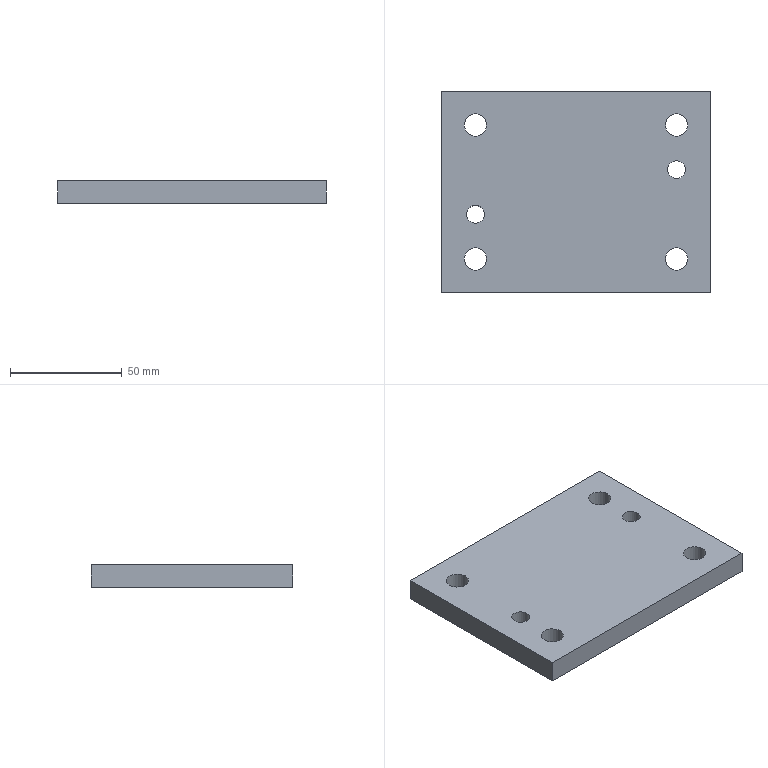Part | NX | features DATUM_CSYS 1, EXTRUDE 1 | 1 solid | 12 faces | box 120 x 90 x 10 mm | volume 103853 mm3 | plane 6 | cylinder 6 | commonest cylinder face diameters 10 x4 8 x2
STEP:
#1=CARTESIAN_POINT('',(60.,-45.,0.));
#2=VERTEX_POINT('',#1);
#3=CARTESIAN_POINT('',(60.,45.,0.));
#4=VERTEX_POINT('',#3);
#5=CARTESIAN_POINT('',(60.,-45.,0.));
#6=DIRECTION('',(0.,1.,0.));
#7=VECTOR('',#6,1000.);
#8=LINE('',#5,#7);
#9=EDGE_CURVE('',#2,#4,#8,.T.);
#10=ORIENTED_EDGE('',*,*,#9,.T.);
#11=CARTESIAN_POINT('',(60.,45.,10.));
#12=VERTEX_POINT('',#11);
#13=CARTESIAN_POINT('',(60.,45.,10.));
#14=DIRECTION('',(0.,0.,-1.));
#15=VECTOR('',#14,1000.);
#16=LINE('',#13,#15);
#17=EDGE_CURVE('',#12,#4,#16,.T.);
#18=ORIENTED_EDGE('',*,*,#17,.F.);
#19=CARTESIAN_POINT('',(60.,-45.,10.));
#20=VERTEX_POINT('',#19);
#21=CARTESIAN_POINT('',(60.,-45.,10.));
#22=DIRECTION('',(0.,1.,0.));
#23=VECTOR('',#22,1000.);
#24=LINE('',#21,#23);
#25=EDGE_CURVE('',#20,#12,#24,.T.);
#26=ORIENTED_EDGE('',*,*,#25,.F.);
#27=CARTESIAN_POINT('',(60.,-45.,10.));
#28=DIRECTION('',(0.,0.,-1.));
#29=VECTOR('',#28,1000.);
#30=LINE('',#27,#29);
#31=EDGE_CURVE('',#20,#2,#30,.T.);
#32=ORIENTED_EDGE('',*,*,#31,.T.);
#33=EDGE_LOOP('',(#10,#18,#26,#32));
#34=FACE_BOUND('',#33,.T.);
#35=CARTESIAN_POINT('',(60.,-45.,10.));
#36=DIRECTION('',(-1.,0.,0.));
#37=DIRECTION('',(0.,0.,1.));
#38=AXIS2_PLACEMENT_3D('',#35,#36,#37);
#39=PLANE('',#38);
#40=ADVANCED_FACE('',(#34),#39,.F.);
#41=CARTESIAN_POINT('',(-60.,45.,0.));
#42=VERTEX_POINT('',#41);
#43=CARTESIAN_POINT('',(60.,45.,0.));
#44=DIRECTION('',(-1.,0.,0.));
#45=VECTOR('',#44,1000.);
#46=LINE('',#43,#45);
#47=EDGE_CURVE('',#4,#42,#46,.T.);
#48=ORIENTED_EDGE('',*,*,#47,.T.);
#49=CARTESIAN_POINT('',(-60.,45.,10.));
#50=VERTEX_POINT('',#49);
#51=CARTESIAN_POINT('',(-60.,45.,10.));
#52=DIRECTION('',(0.,0.,-1.));
#53=VECTOR('',#52,1000.);
#54=LINE('',#51,#53);
#55=EDGE_CURVE('',#50,#42,#54,.T.);
#56=ORIENTED_EDGE('',*,*,#55,.F.);
#57=CARTESIAN_POINT('',(60.,45.,10.));
#58=DIRECTION('',(-1.,0.,0.));
#59=VECTOR('',#58,1000.);
#60=LINE('',#57,#59);
#61=EDGE_CURVE('',#12,#50,#60,.T.);
#62=ORIENTED_EDGE('',*,*,#61,.F.);
#63=ORIENTED_EDGE('',*,*,#17,.T.);
#64=EDGE_LOOP('',(#48,#56,#62,#63));
#65=FACE_BOUND('',#64,.T.);
#66=CARTESIAN_POINT('',(60.,45.,10.));
#67=DIRECTION('',(0.,-1.,0.));
#68=DIRECTION('',(0.,0.,-1.));
#69=AXIS2_PLACEMENT_3D('',#66,#67,#68);
#70=PLANE('',#69);
#71=ADVANCED_FACE('',(#65),#70,.F.);
#72=CARTESIAN_POINT('',(-60.,-45.,0.));
#73=VERTEX_POINT('',#72);
#74=CARTESIAN_POINT('',(-60.,45.,0.));
#75=DIRECTION('',(0.,-1.,0.));
#76=VECTOR('',#75,1000.);
#77=LINE('',#74,#76);
#78=EDGE_CURVE('',#42,#73,#77,.T.);
#79=ORIENTED_EDGE('',*,*,#78,.T.);
#80=CARTESIAN_POINT('',(-60.,-45.,10.));
#81=VERTEX_POINT('',#80);
#82=CARTESIAN_POINT('',(-60.,-45.,10.));
#83=DIRECTION('',(0.,0.,-1.));
#84=VECTOR('',#83,1000.);
#85=LINE('',#82,#84);
#86=EDGE_CURVE('',#81,#73,#85,.T.);
#87=ORIENTED_EDGE('',*,*,#86,.F.);
#88=CARTESIAN_POINT('',(-60.,45.,10.));
#89=DIRECTION('',(0.,-1.,0.));
#90=VECTOR('',#89,1000.);
#91=LINE('',#88,#90);
#92=EDGE_CURVE('',#50,#81,#91,.T.);
#93=ORIENTED_EDGE('',*,*,#92,.F.);
#94=ORIENTED_EDGE('',*,*,#55,.T.);
#95=EDGE_LOOP('',(#79,#87,#93,#94));
#96=FACE_BOUND('',#95,.T.);
#97=CARTESIAN_POINT('',(-60.,45.,10.));
#98=DIRECTION('',(1.,0.,0.));
#99=DIRECTION('',(0.,0.,-1.));
#100=AXIS2_PLACEMENT_3D('',#97,#98,#99);
#101=PLANE('',#100);
#102=ADVANCED_FACE('',(#96),#101,.F.);
#103=CARTESIAN_POINT('',(50.,30.,10.));
#104=VERTEX_POINT('',#103);
#105=CARTESIAN_POINT('',(45.,30.,10.));
#106=DIRECTION('',(0.,0.,1.));
#107=DIRECTION('',(1.,0.,0.));
#108=AXIS2_PLACEMENT_3D('',#105,#106,#107);
#109=CIRCLE('',#108,5.);
#110=EDGE_CURVE('',#104,#104,#109,.T.);
#111=ORIENTED_EDGE('',*,*,#110,.T.);
#112=EDGE_LOOP('',(#111));
#113=FACE_BOUND('',#112,.T.);
#114=CARTESIAN_POINT('',(50.,30.,0.));
#115=VERTEX_POINT('',#114);
#116=CARTESIAN_POINT('',(45.,30.,0.));
#117=DIRECTION('',(0.,0.,1.));
#118=DIRECTION('',(1.,0.,0.));
#119=AXIS2_PLACEMENT_3D('',#116,#117,#118);
#120=CIRCLE('',#119,5.);
#121=EDGE_CURVE('',#115,#115,#120,.T.);
#122=ORIENTED_EDGE('',*,*,#121,.F.);
#123=EDGE_LOOP('',(#122));
#124=FACE_BOUND('',#123,.T.);
#125=CARTESIAN_POINT('',(45.,30.,10.));
#126=DIRECTION('',(0.,0.,-1.));
#127=DIRECTION('',(-1.,0.,0.));
#128=AXIS2_PLACEMENT_3D('',#125,#126,#127);
#129=CYLINDRICAL_SURFACE('',#128,5.);
#130=ADVANCED_FACE('',(#113,#124),#129,.F.);
#131=CARTESIAN_POINT('',(50.,-30.,10.));
#132=VERTEX_POINT('',#131);
#133=CARTESIAN_POINT('',(45.,-30.,10.));
#134=DIRECTION('',(0.,0.,1.));
#135=DIRECTION('',(1.,0.,0.));
#136=AXIS2_PLACEMENT_3D('',#133,#134,#135);
#137=CIRCLE('',#136,5.);
#138=EDGE_CURVE('',#132,#132,#137,.T.);
#139=ORIENTED_EDGE('',*,*,#138,.T.);
#140=EDGE_LOOP('',(#139));
#141=FACE_BOUND('',#140,.T.);
#142=CARTESIAN_POINT('',(50.,-30.,0.));
#143=VERTEX_POINT('',#142);
#144=CARTESIAN_POINT('',(45.,-30.,0.));
#145=DIRECTION('',(0.,0.,1.));
#146=DIRECTION('',(1.,0.,0.));
#147=AXIS2_PLACEMENT_3D('',#144,#145,#146);
#148=CIRCLE('',#147,5.);
#149=EDGE_CURVE('',#143,#143,#148,.T.);
#150=ORIENTED_EDGE('',*,*,#149,.F.);
#151=EDGE_LOOP('',(#150));
#152=FACE_BOUND('',#151,.T.);
#153=CARTESIAN_POINT('',(45.,-30.,10.));
#154=DIRECTION('',(0.,0.,-1.));
#155=DIRECTION('',(-1.,0.,0.));
#156=AXIS2_PLACEMENT_3D('',#153,#154,#155);
#157=CYLINDRICAL_SURFACE('',#156,5.);
#158=ADVANCED_FACE('',(#141,#152),#157,.F.);
#159=CARTESIAN_POINT('',(-41.,-10.,10.));
#160=VERTEX_POINT('',#159);
#161=CARTESIAN_POINT('',(-45.,-10.,10.));
#162=DIRECTION('',(0.,0.,1.));
#163=DIRECTION('',(1.,0.,0.));
#164=AXIS2_PLACEMENT_3D('',#161,#162,#163);
#165=CIRCLE('',#164,4.);
#166=EDGE_CURVE('',#160,#160,#165,.T.);
#167=ORIENTED_EDGE('',*,*,#166,.T.);
#168=EDGE_LOOP('',(#167));
#169=FACE_BOUND('',#168,.T.);
#170=CARTESIAN_POINT('',(-41.,-10.,0.));
#171=VERTEX_POINT('',#170);
#172=CARTESIAN_POINT('',(-45.,-10.,0.));
#173=DIRECTION('',(0.,0.,1.));
#174=DIRECTION('',(1.,0.,0.));
#175=AXIS2_PLACEMENT_3D('',#172,#173,#174);
#176=CIRCLE('',#175,4.);
#177=EDGE_CURVE('',#171,#171,#176,.T.);
#178=ORIENTED_EDGE('',*,*,#177,.F.);
#179=EDGE_LOOP('',(#178));
#180=FACE_BOUND('',#179,.T.);
#181=CARTESIAN_POINT('',(-45.,-10.,10.));
#182=DIRECTION('',(0.,0.,-1.));
#183=DIRECTION('',(-1.,0.,0.));
#184=AXIS2_PLACEMENT_3D('',#181,#182,#183);
#185=CYLINDRICAL_SURFACE('',#184,4.);
#186=ADVANCED_FACE('',(#169,#180),#185,.F.);
#187=CARTESIAN_POINT('',(-40.,30.,10.));
#188=VERTEX_POINT('',#187);
#189=CARTESIAN_POINT('',(-45.,30.,10.));
#190=DIRECTION('',(0.,0.,1.));
#191=DIRECTION('',(1.,0.,0.));
#192=AXIS2_PLACEMENT_3D('',#189,#190,#191);
#193=CIRCLE('',#192,5.);
#194=EDGE_CURVE('',#188,#188,#193,.T.);
#195=ORIENTED_EDGE('',*,*,#194,.T.);
#196=EDGE_LOOP('',(#195));
#197=FACE_BOUND('',#196,.T.);
#198=CARTESIAN_POINT('',(-40.,30.,0.));
#199=VERTEX_POINT('',#198);
#200=CARTESIAN_POINT('',(-45.,30.,0.));
#201=DIRECTION('',(0.,0.,1.));
#202=DIRECTION('',(1.,0.,0.));
#203=AXIS2_PLACEMENT_3D('',#200,#201,#202);
#204=CIRCLE('',#203,5.);
#205=EDGE_CURVE('',#199,#199,#204,.T.);
#206=ORIENTED_EDGE('',*,*,#205,.F.);
#207=EDGE_LOOP('',(#206));
#208=FACE_BOUND('',#207,.T.);
#209=CARTESIAN_POINT('',(-45.,30.,10.));
#210=DIRECTION('',(0.,0.,-1.));
#211=DIRECTION('',(-1.,0.,0.));
#212=AXIS2_PLACEMENT_3D('',#209,#210,#211);
#213=CYLINDRICAL_SURFACE('',#212,5.);
#214=ADVANCED_FACE('',(#197,#208),#213,.F.);
#215=CARTESIAN_POINT('',(-40.,-30.,10.));
#216=VERTEX_POINT('',#215);
#217=CARTESIAN_POINT('',(-45.,-30.,10.));
#218=DIRECTION('',(0.,0.,1.));
#219=DIRECTION('',(1.,0.,0.));
#220=AXIS2_PLACEMENT_3D('',#217,#218,#219);
#221=CIRCLE('',#220,5.);
#222=EDGE_CURVE('',#216,#216,#221,.T.);
#223=ORIENTED_EDGE('',*,*,#222,.T.);
#224=EDGE_LOOP('',(#223));
#225=FACE_BOUND('',#224,.T.);
#226=CARTESIAN_POINT('',(-40.,-30.,0.));
#227=VERTEX_POINT('',#226);
#228=CARTESIAN_POINT('',(-45.,-30.,0.));
#229=DIRECTION('',(0.,0.,1.));
#230=DIRECTION('',(1.,0.,0.));
#231=AXIS2_PLACEMENT_3D('',#228,#229,#230);
#232=CIRCLE('',#231,5.);
#233=EDGE_CURVE('',#227,#227,#232,.T.);
#234=ORIENTED_EDGE('',*,*,#233,.F.);
#235=EDGE_LOOP('',(#234));
#236=FACE_BOUND('',#235,.T.);
#237=CARTESIAN_POINT('',(-45.,-30.,10.));
#238=DIRECTION('',(0.,0.,-1.));
#239=DIRECTION('',(-1.,0.,0.));
#240=AXIS2_PLACEMENT_3D('',#237,#238,#239);
#241=CYLINDRICAL_SURFACE('',#240,5.);
#242=ADVANCED_FACE('',(#225,#236),#241,.F.);
#243=CARTESIAN_POINT('',(-60.,-45.,0.));
#244=DIRECTION('',(1.,0.,0.));
#245=VECTOR('',#244,1000.);
#246=LINE('',#243,#245);
#247=EDGE_CURVE('',#73,#2,#246,.T.);
#248=ORIENTED_EDGE('',*,*,#247,.T.);
#249=ORIENTED_EDGE('',*,*,#31,.F.);
#250=CARTESIAN_POINT('',(-60.,-45.,10.));
#251=DIRECTION('',(1.,0.,0.));
#252=VECTOR('',#251,1000.);
#253=LINE('',#250,#252);
#254=EDGE_CURVE('',#81,#20,#253,.T.);
#255=ORIENTED_EDGE('',*,*,#254,.F.);
#256=ORIENTED_EDGE('',*,*,#86,.T.);
#257=EDGE_LOOP('',(#248,#249,#255,#256));
#258=FACE_BOUND('',#257,.T.);
#259=CARTESIAN_POINT('',(-60.,-45.,10.));
#260=DIRECTION('',(0.,1.,0.));
#261=DIRECTION('',(0.,0.,1.));
#262=AXIS2_PLACEMENT_3D('',#259,#260,#261);
#263=PLANE('',#262);
#264=ADVANCED_FACE('',(#258),#263,.F.);
#265=CARTESIAN_POINT('',(49.,10.,10.));
#266=VERTEX_POINT('',#265);
#267=CARTESIAN_POINT('',(45.,10.,10.));
#268=DIRECTION('',(0.,0.,1.));
#269=DIRECTION('',(1.,0.,0.));
#270=AXIS2_PLACEMENT_3D('',#267,#268,#269);
#271=CIRCLE('',#270,4.);
#272=EDGE_CURVE('',#266,#266,#271,.T.);
#273=ORIENTED_EDGE('',*,*,#272,.T.);
#274=EDGE_LOOP('',(#273));
#275=FACE_BOUND('',#274,.T.);
#276=CARTESIAN_POINT('',(49.,10.,0.));
#277=VERTEX_POINT('',#276);
#278=CARTESIAN_POINT('',(45.,10.,0.));
#279=DIRECTION('',(0.,0.,1.));
#280=DIRECTION('',(1.,0.,0.));
#281=AXIS2_PLACEMENT_3D('',#278,#279,#280);
#282=CIRCLE('',#281,4.);
#283=EDGE_CURVE('',#277,#277,#282,.T.);
#284=ORIENTED_EDGE('',*,*,#283,.F.);
#285=EDGE_LOOP('',(#284));
#286=FACE_BOUND('',#285,.T.);
#287=CARTESIAN_POINT('',(45.,10.,10.));
#288=DIRECTION('',(0.,0.,-1.));
#289=DIRECTION('',(-1.,0.,0.));
#290=AXIS2_PLACEMENT_3D('',#287,#288,#289);
#291=CYLINDRICAL_SURFACE('',#290,4.);
#292=ADVANCED_FACE('',(#275,#286),#291,.F.);
#293=ORIENTED_EDGE('',*,*,#25,.T.);
#294=ORIENTED_EDGE('',*,*,#61,.T.);
#295=ORIENTED_EDGE('',*,*,#92,.T.);
#296=ORIENTED_EDGE('',*,*,#254,.T.);
#297=EDGE_LOOP('',(#293,#294,#295,#296));
#298=FACE_BOUND('',#297,.T.);
#299=ORIENTED_EDGE('',*,*,#222,.F.);
#300=EDGE_LOOP('',(#299));
#301=FACE_BOUND('',#300,.T.);
#302=ORIENTED_EDGE('',*,*,#194,.F.);
#303=EDGE_LOOP('',(#302));
#304=FACE_BOUND('',#303,.T.);
#305=ORIENTED_EDGE('',*,*,#166,.F.);
#306=EDGE_LOOP('',(#305));
#307=FACE_BOUND('',#306,.T.);
#308=ORIENTED_EDGE('',*,*,#138,.F.);
#309=EDGE_LOOP('',(#308));
#310=FACE_BOUND('',#309,.T.);
#311=ORIENTED_EDGE('',*,*,#110,.F.);
#312=EDGE_LOOP('',(#311));
#313=FACE_BOUND('',#312,.T.);
#314=ORIENTED_EDGE('',*,*,#272,.F.);
#315=EDGE_LOOP('',(#314));
#316=FACE_BOUND('',#315,.T.);
#317=CARTESIAN_POINT('',(-45.,-30.,10.));
#318=DIRECTION('',(0.,0.,1.));
#319=DIRECTION('',(1.,0.,0.));
#320=AXIS2_PLACEMENT_3D('',#317,#318,#319);
#321=PLANE('',#320);
#322=ADVANCED_FACE('',(#298,#301,#304,#307,#310,#313,#316),#321,.T.);
#323=ORIENTED_EDGE('',*,*,#9,.F.);
#324=ORIENTED_EDGE('',*,*,#247,.F.);
#325=ORIENTED_EDGE('',*,*,#78,.F.);
#326=ORIENTED_EDGE('',*,*,#47,.F.);
#327=EDGE_LOOP('',(#323,#324,#325,#326));
#328=FACE_BOUND('',#327,.T.);
#329=ORIENTED_EDGE('',*,*,#233,.T.);
#330=EDGE_LOOP('',(#329));
#331=FACE_BOUND('',#330,.T.);
#332=ORIENTED_EDGE('',*,*,#205,.T.);
#333=EDGE_LOOP('',(#332));
#334=FACE_BOUND('',#333,.T.);
#335=ORIENTED_EDGE('',*,*,#177,.T.);
#336=EDGE_LOOP('',(#335));
#337=FACE_BOUND('',#336,.T.);
#338=ORIENTED_EDGE('',*,*,#149,.T.);
#339=EDGE_LOOP('',(#338));
#340=FACE_BOUND('',#339,.T.);
#341=ORIENTED_EDGE('',*,*,#121,.T.);
#342=EDGE_LOOP('',(#341));
#343=FACE_BOUND('',#342,.T.);
#344=ORIENTED_EDGE('',*,*,#283,.T.);
#345=EDGE_LOOP('',(#344));
#346=FACE_BOUND('',#345,.T.);
#347=CARTESIAN_POINT('',(-45.,-30.,0.));
#348=DIRECTION('',(0.,0.,1.));
#349=DIRECTION('',(1.,0.,0.));
#350=AXIS2_PLACEMENT_3D('',#347,#348,#349);
#351=PLANE('',#350);
#352=ADVANCED_FACE('',(#328,#331,#334,#337,#340,#343,#346),#351,.F.);
#353=CLOSED_SHELL('',(#40,#71,#102,#130,#158,#186,#214,#242,#264,#292,#322,#352));
#354=MANIFOLD_SOLID_BREP('',#353);
#355=(LENGTH_UNIT()NAMED_UNIT(*)SI_UNIT(.MILLI.,.METRE.));
#356=UNCERTAINTY_MEASURE_WITH_UNIT(LENGTH_MEASURE(0.00001),#355,'','');
#357=(NAMED_UNIT(*)PLANE_ANGLE_UNIT()SI_UNIT($,.RADIAN.));
#358=(NAMED_UNIT(*)SI_UNIT($,.STERADIAN.)SOLID_ANGLE_UNIT());
#359=(GEOMETRIC_REPRESENTATION_CONTEXT(3)GLOBAL_UNCERTAINTY_ASSIGNED_CONTEXT((#356))GLOBAL_UNIT_ASSIGNED_CONTEXT((#355,#357,#358))REPRESENTATION_CONTEXT('',''));
#360=ADVANCED_BREP_SHAPE_REPRESENTATION('',(#354),#359);